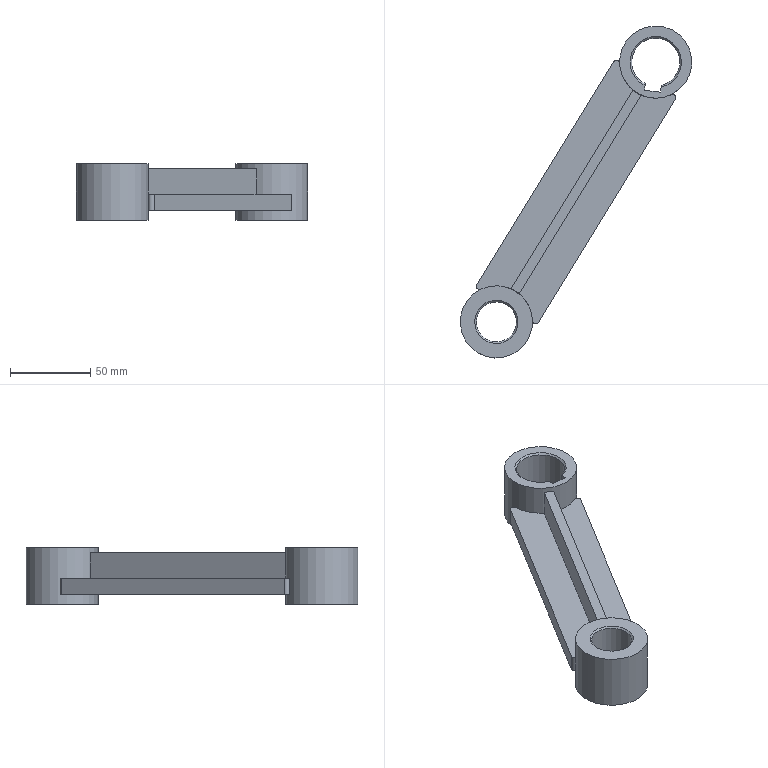Part | STEP file | HL4GZ-1.313.024 (upper steering tie-rod weldment) | 4 solids | 31 faces | box 144.341 x 206.961 x 35 mm | volume 151003 mm3 | plane 17 | cylinder 10 | cone 4 | commonest cylinder face diameters 4 x4 45 x4 25 x1 30 x1